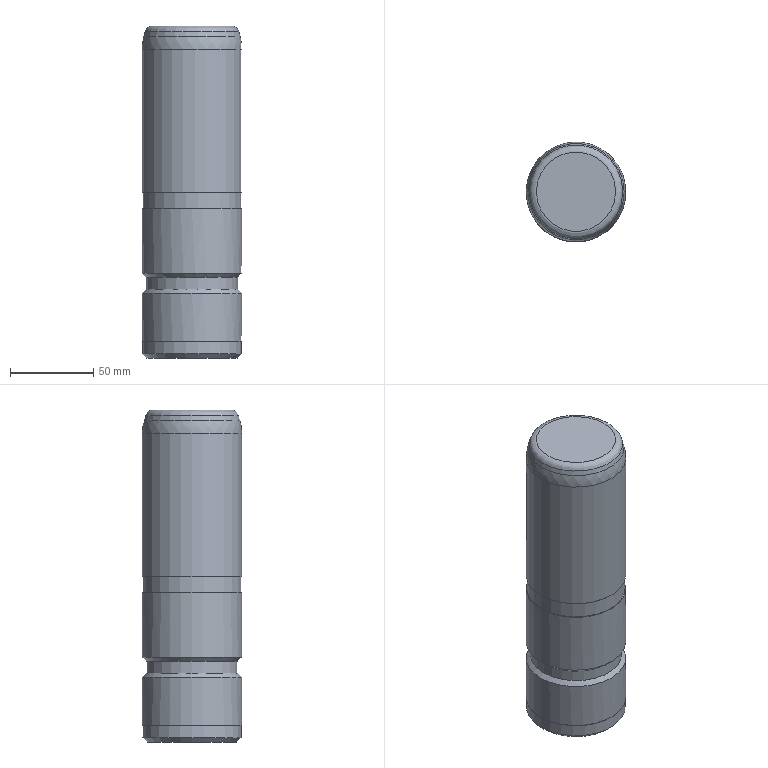Part | NX | features solid 2 | 1 solid | 17 faces | box 60 x 60 x 200 mm | volume 556247 mm3 | cylinder 6 | plane 5 | cone 4 | sphere 1 | torus 1 | commonest cylinder face diameters 60 x3 55 x1 59 x1 59.5 x1
STEP:
#1=CARTESIAN_POINT('',(1295.,185.,-349.));
#2=VERTEX_POINT('',#1);
#3=CARTESIAN_POINT('',(1325.,185.,-349.));
#4=DIRECTION('',(0.,0.,-1.));
#5=DIRECTION('',(-1.,0.,0.));
#6=AXIS2_PLACEMENT_3D('',#3,#4,#5);
#7=CIRCLE('',#6,30.);
#8=EDGE_CURVE('',#2,#2,#7,.F.);
#9=ORIENTED_EDGE('',*,*,#8,.T.);
#10=EDGE_LOOP('',(#9));
#11=FACE_BOUND('',#10,.T.);
#12=CARTESIAN_POINT('',(1355.,185.,-310.));
#13=VERTEX_POINT('',#12);
#14=CARTESIAN_POINT('',(1325.,185.,-310.));
#15=DIRECTION('',(0.,0.,1.));
#16=DIRECTION('',(1.,0.,0.));
#17=AXIS2_PLACEMENT_3D('',#14,#15,#16);
#18=CIRCLE('',#17,30.);
#19=EDGE_CURVE('',#13,#13,#18,.T.);
#20=ORIENTED_EDGE('',*,*,#19,.F.);
#21=EDGE_LOOP('',(#20));
#22=FACE_BOUND('',#21,.T.);
#23=CARTESIAN_POINT('',(1325.,185.,-390.));
#24=DIRECTION('',(0.,0.,1.));
#25=DIRECTION('',(-1.,0.,0.));
#26=AXIS2_PLACEMENT_3D('',#23,#24,#25);
#27=CYLINDRICAL_SURFACE('',#26,30.);
#28=ADVANCED_FACE('',(#11,#22),#27,.T.);
#29=CARTESIAN_POINT('',(1295.5,185.,-310.));
#30=VERTEX_POINT('',#29);
#31=CARTESIAN_POINT('',(1325.,185.,-310.));
#32=DIRECTION('',(0.,0.,-1.));
#33=DIRECTION('',(-1.,0.,0.));
#34=AXIS2_PLACEMENT_3D('',#31,#32,#33);
#35=CIRCLE('',#34,29.5);
#36=EDGE_CURVE('',#30,#30,#35,.T.);
#37=ORIENTED_EDGE('',*,*,#36,.T.);
#38=EDGE_LOOP('',(#37));
#39=FACE_BOUND('',#38,.T.);
#40=ORIENTED_EDGE('',*,*,#19,.T.);
#41=EDGE_LOOP('',(#40));
#42=FACE_BOUND('',#41,.T.);
#43=CARTESIAN_POINT('',(1325.,185.,-310.));
#44=DIRECTION('',(0.,0.,1.));
#45=DIRECTION('',(-1.,0.,0.));
#46=AXIS2_PLACEMENT_3D('',#43,#44,#45);
#47=PLANE('',#46);
#48=ADVANCED_FACE('',(#39,#42),#47,.T.);
#49=CARTESIAN_POINT('',(1354.5,185.,-300.));
#50=VERTEX_POINT('',#49);
#51=CARTESIAN_POINT('',(1325.,185.,-300.));
#52=DIRECTION('',(0.,0.,1.));
#53=DIRECTION('',(1.,0.,0.));
#54=AXIS2_PLACEMENT_3D('',#51,#52,#53);
#55=CIRCLE('',#54,29.5);
#56=EDGE_CURVE('',#50,#50,#55,.F.);
#57=ORIENTED_EDGE('',*,*,#56,.T.);
#58=EDGE_LOOP('',(#57));
#59=FACE_BOUND('',#58,.T.);
#60=ORIENTED_EDGE('',*,*,#36,.F.);
#61=EDGE_LOOP('',(#60));
#62=FACE_BOUND('',#61,.T.);
#63=CARTESIAN_POINT('',(1325.,185.,-310.));
#64=DIRECTION('',(0.,0.,1.));
#65=DIRECTION('',(-1.,0.,0.));
#66=AXIS2_PLACEMENT_3D('',#63,#64,#65);
#67=CYLINDRICAL_SURFACE('',#66,29.5);
#68=ADVANCED_FACE('',(#59,#62),#67,.T.);
#69=ORIENTED_EDGE('',*,*,#56,.F.);
#70=EDGE_LOOP('',(#69));
#71=FACE_BOUND('',#70,.T.);
#72=CARTESIAN_POINT('',(1295.,185.,-300.));
#73=VERTEX_POINT('',#72);
#74=CARTESIAN_POINT('',(1325.,185.,-300.));
#75=DIRECTION('',(0.,0.,-1.));
#76=DIRECTION('',(-1.,0.,0.));
#77=AXIS2_PLACEMENT_3D('',#74,#75,#76);
#78=CIRCLE('',#77,30.);
#79=EDGE_CURVE('',#73,#73,#78,.T.);
#80=ORIENTED_EDGE('',*,*,#79,.T.);
#81=EDGE_LOOP('',(#80));
#82=FACE_BOUND('',#81,.T.);
#83=CARTESIAN_POINT('',(1325.,185.,-300.));
#84=DIRECTION('',(0.,0.,-1.));
#85=DIRECTION('',(1.,0.,0.));
#86=AXIS2_PLACEMENT_3D('',#83,#84,#85);
#87=PLANE('',#86);
#88=ADVANCED_FACE('',(#71,#82),#87,.T.);
#89=CARTESIAN_POINT('',(1295.,185.,-213.95));
#90=VERTEX_POINT('',#89);
#91=CARTESIAN_POINT('',(1325.,185.,-213.95));
#92=DIRECTION('',(0.,0.,-1.));
#93=DIRECTION('',(-1.,0.,0.));
#94=AXIS2_PLACEMENT_3D('',#91,#92,#93);
#95=CIRCLE('',#94,30.);
#96=EDGE_CURVE('',#90,#90,#95,.F.);
#97=ORIENTED_EDGE('',*,*,#96,.F.);
#98=EDGE_LOOP('',(#97));
#99=FACE_BOUND('',#98,.T.);
#100=ORIENTED_EDGE('',*,*,#79,.F.);
#101=EDGE_LOOP('',(#100));
#102=FACE_BOUND('',#101,.T.);
#103=CARTESIAN_POINT('',(1325.,185.,-300.));
#104=DIRECTION('',(0.,0.,1.));
#105=DIRECTION('',(-1.,0.,0.));
#106=AXIS2_PLACEMENT_3D('',#103,#104,#105);
#107=CYLINDRICAL_SURFACE('',#106,30.);
#108=ADVANCED_FACE('',(#99,#102),#107,.T.);
#109=CARTESIAN_POINT('',(1301.132,185.,-200.));
#110=VERTEX_POINT('',#109);
#111=CARTESIAN_POINT('',(1325.,185.,-200.));
#112=DIRECTION('',(0.,0.,-1.));
#113=DIRECTION('',(-1.,0.,0.));
#114=AXIS2_PLACEMENT_3D('',#111,#112,#113);
#115=CIRCLE('',#114,23.868);
#116=EDGE_CURVE('',#110,#110,#115,.T.);
#117=ORIENTED_EDGE('',*,*,#116,.F.);
#118=EDGE_LOOP('',(#117));
#119=FACE_BOUND('',#118,.T.);
#120=CARTESIAN_POINT('',(1325.,185.,-200.));
#121=DIRECTION('',(0.,0.,1.));
#122=DIRECTION('',(-1.,0.,0.));
#123=AXIS2_PLACEMENT_3D('',#120,#121,#122);
#124=PLANE('',#123);
#125=ADVANCED_FACE('',(#119),#124,.T.);
#126=CARTESIAN_POINT('',(1296.786,185.,-203.335));
#127=VERTEX_POINT('',#126);
#128=CARTESIAN_POINT('',(1325.,185.,-203.335));
#129=DIRECTION('',(0.,0.,-1.));
#130=DIRECTION('',(-1.,0.,0.));
#131=AXIS2_PLACEMENT_3D('',#128,#129,#130);
#132=CIRCLE('',#131,28.214);
#133=EDGE_CURVE('',#127,#127,#132,.F.);
#134=ORIENTED_EDGE('',*,*,#133,.F.);
#135=EDGE_LOOP('',(#134));
#136=FACE_BOUND('',#135,.T.);
#137=CARTESIAN_POINT('',(1353.978,185.,-206.185));
#138=VERTEX_POINT('',#137);
#139=CARTESIAN_POINT('',(1325.,185.,-206.185));
#140=DIRECTION('',(0.,0.,1.));
#141=DIRECTION('',(1.,0.,0.));
#142=AXIS2_PLACEMENT_3D('',#139,#140,#141);
#143=CIRCLE('',#142,28.978);
#144=EDGE_CURVE('',#138,#138,#143,.F.);
#145=ORIENTED_EDGE('',*,*,#144,.F.);
#146=EDGE_LOOP('',(#145));
#147=FACE_BOUND('',#146,.T.);
#148=CARTESIAN_POINT('',(1325.,185.,-200.));
#149=DIRECTION('',(0.,0.,-1.));
#150=DIRECTION('',(1.,0.,0.));
#151=AXIS2_PLACEMENT_3D('',#148,#149,#150);
#152=CONICAL_SURFACE('',#151,27.321,0.2618);
#153=ADVANCED_FACE('',(#136,#147),#152,.T.);
#154=CARTESIAN_POINT('',(1297.5,185.,-351.5));
#155=VERTEX_POINT('',#154);
#156=CARTESIAN_POINT('',(1325.,185.,-351.5));
#157=DIRECTION('',(0.,0.,-1.));
#158=DIRECTION('',(-1.,0.,0.));
#159=AXIS2_PLACEMENT_3D('',#156,#157,#158);
#160=CIRCLE('',#159,27.5);
#161=EDGE_CURVE('',#155,#155,#160,.F.);
#162=ORIENTED_EDGE('',*,*,#161,.F.);
#163=EDGE_LOOP('',(#162));
#164=FACE_BOUND('',#163,.T.);
#165=CARTESIAN_POINT('',(1352.5,185.,-358.5));
#166=VERTEX_POINT('',#165);
#167=CARTESIAN_POINT('',(1325.,185.,-358.5));
#168=DIRECTION('',(0.,0.,1.));
#169=DIRECTION('',(1.,0.,0.));
#170=AXIS2_PLACEMENT_3D('',#167,#168,#169);
#171=CIRCLE('',#170,27.5);
#172=EDGE_CURVE('',#166,#166,#171,.F.);
#173=ORIENTED_EDGE('',*,*,#172,.F.);
#174=EDGE_LOOP('',(#173));
#175=FACE_BOUND('',#174,.T.);
#176=CARTESIAN_POINT('',(1325.,185.,-361.));
#177=DIRECTION('',(0.,0.,1.));
#178=DIRECTION('',(-1.,0.,0.));
#179=AXIS2_PLACEMENT_3D('',#176,#177,#178);
#180=CYLINDRICAL_SURFACE('',#179,27.5);
#181=ADVANCED_FACE('',(#164,#175),#180,.T.);
#182=CARTESIAN_POINT('',(1352.25,185.,-400.));
#183=VERTEX_POINT('',#182);
#184=CARTESIAN_POINT('',(1325.,185.,-400.));
#185=DIRECTION('',(0.,0.,1.));
#186=DIRECTION('',(1.,0.,0.));
#187=AXIS2_PLACEMENT_3D('',#184,#185,#186);
#188=CIRCLE('',#187,27.25);
#189=EDGE_CURVE('',#183,#183,#188,.T.);
#190=ORIENTED_EDGE('',*,*,#189,.F.);
#191=EDGE_LOOP('',(#190));
#192=FACE_BOUND('',#191,.T.);
#193=CARTESIAN_POINT('',(1325.,185.,-400.));
#194=DIRECTION('',(0.,0.,-1.));
#195=DIRECTION('',(1.,0.,0.));
#196=AXIS2_PLACEMENT_3D('',#193,#194,#195);
#197=PLANE('',#196);
#198=ADVANCED_FACE('',(#192),#197,.T.);
#199=CARTESIAN_POINT('',(1354.75,185.,-397.5));
#200=VERTEX_POINT('',#199);
#201=CARTESIAN_POINT('',(1325.,185.,-397.5));
#202=DIRECTION('',(0.,0.,1.));
#203=DIRECTION('',(1.,0.,0.));
#204=AXIS2_PLACEMENT_3D('',#201,#202,#203);
#205=CIRCLE('',#204,29.75);
#206=EDGE_CURVE('',#200,#200,#205,.F.);
#207=ORIENTED_EDGE('',*,*,#206,.F.);
#208=EDGE_LOOP('',(#207));
#209=FACE_BOUND('',#208,.T.);
#210=CARTESIAN_POINT('',(1354.75,185.,-390.));
#211=VERTEX_POINT('',#210);
#212=CARTESIAN_POINT('',(1325.,185.,-390.));
#213=DIRECTION('',(0.,0.,1.));
#214=DIRECTION('',(1.,0.,0.));
#215=AXIS2_PLACEMENT_3D('',#212,#213,#214);
#216=CIRCLE('',#215,29.75);
#217=EDGE_CURVE('',#211,#211,#216,.F.);
#218=ORIENTED_EDGE('',*,*,#217,.T.);
#219=EDGE_LOOP('',(#218));
#220=FACE_BOUND('',#219,.T.);
#221=CARTESIAN_POINT('',(1325.,185.,-400.));
#222=DIRECTION('',(0.,0.,1.));
#223=DIRECTION('',(-1.,0.,0.));
#224=AXIS2_PLACEMENT_3D('',#221,#222,#223);
#225=CYLINDRICAL_SURFACE('',#224,29.75);
#226=ADVANCED_FACE('',(#209,#220),#225,.T.);
#227=ORIENTED_EDGE('',*,*,#217,.F.);
#228=EDGE_LOOP('',(#227));
#229=FACE_BOUND('',#228,.T.);
#230=CARTESIAN_POINT('',(1295.,185.,-390.));
#231=VERTEX_POINT('',#230);
#232=CARTESIAN_POINT('',(1325.,185.,-390.));
#233=DIRECTION('',(0.,0.,-1.));
#234=DIRECTION('',(-1.,0.,0.));
#235=AXIS2_PLACEMENT_3D('',#232,#233,#234);
#236=CIRCLE('',#235,30.);
#237=EDGE_CURVE('',#231,#231,#236,.T.);
#238=ORIENTED_EDGE('',*,*,#237,.T.);
#239=EDGE_LOOP('',(#238));
#240=FACE_BOUND('',#239,.T.);
#241=CARTESIAN_POINT('',(1325.,185.,-390.));
#242=DIRECTION('',(0.,0.,-1.));
#243=DIRECTION('',(1.,0.,0.));
#244=AXIS2_PLACEMENT_3D('',#241,#242,#243);
#245=PLANE('',#244);
#246=ADVANCED_FACE('',(#229,#240),#245,.T.);
#247=CARTESIAN_POINT('',(1355.,185.,-361.));
#248=VERTEX_POINT('',#247);
#249=CARTESIAN_POINT('',(1325.,185.,-361.));
#250=DIRECTION('',(0.,0.,1.));
#251=DIRECTION('',(1.,0.,0.));
#252=AXIS2_PLACEMENT_3D('',#249,#250,#251);
#253=CIRCLE('',#252,30.);
#254=EDGE_CURVE('',#248,#248,#253,.F.);
#255=ORIENTED_EDGE('',*,*,#254,.T.);
#256=EDGE_LOOP('',(#255));
#257=FACE_BOUND('',#256,.T.);
#258=ORIENTED_EDGE('',*,*,#237,.F.);
#259=EDGE_LOOP('',(#258));
#260=FACE_BOUND('',#259,.T.);
#261=CARTESIAN_POINT('',(1325.,185.,-390.));
#262=DIRECTION('',(0.,0.,1.));
#263=DIRECTION('',(-1.,0.,0.));
#264=AXIS2_PLACEMENT_3D('',#261,#262,#263);
#265=CYLINDRICAL_SURFACE('',#264,30.);
#266=ADVANCED_FACE('',(#257,#260),#265,.T.);
#267=ORIENTED_EDGE('',*,*,#189,.T.);
#268=EDGE_LOOP('',(#267));
#269=FACE_BOUND('',#268,.T.);
#270=ORIENTED_EDGE('',*,*,#206,.T.);
#271=EDGE_LOOP('',(#270));
#272=FACE_BOUND('',#271,.T.);
#273=CARTESIAN_POINT('',(1325.,185.,-397.5));
#274=DIRECTION('',(0.,0.,1.));
#275=DIRECTION('',(-1.,0.,0.));
#276=AXIS2_PLACEMENT_3D('',#273,#274,#275);
#277=CONICAL_SURFACE('',#276,29.75,0.7854);
#278=ADVANCED_FACE('',(#269,#272),#277,.T.);
#279=ORIENTED_EDGE('',*,*,#254,.F.);
#280=EDGE_LOOP('',(#279));
#281=FACE_BOUND('',#280,.T.);
#282=ORIENTED_EDGE('',*,*,#172,.T.);
#283=EDGE_LOOP('',(#282));
#284=FACE_BOUND('',#283,.T.);
#285=CARTESIAN_POINT('',(1325.,185.,-358.5));
#286=DIRECTION('',(0.,0.,-1.));
#287=DIRECTION('',(1.,0.,0.));
#288=AXIS2_PLACEMENT_3D('',#285,#286,#287);
#289=CONICAL_SURFACE('',#288,27.5,0.7854);
#290=ADVANCED_FACE('',(#281,#284),#289,.T.);
#291=ORIENTED_EDGE('',*,*,#8,.F.);
#292=EDGE_LOOP('',(#291));
#293=FACE_BOUND('',#292,.T.);
#294=ORIENTED_EDGE('',*,*,#161,.T.);
#295=EDGE_LOOP('',(#294));
#296=FACE_BOUND('',#295,.T.);
#297=CARTESIAN_POINT('',(1325.,185.,-351.5));
#298=DIRECTION('',(0.,0.,1.));
#299=DIRECTION('',(-1.,0.,0.));
#300=AXIS2_PLACEMENT_3D('',#297,#298,#299);
#301=CONICAL_SURFACE('',#300,27.5,0.7854);
#302=ADVANCED_FACE('',(#293,#296),#301,.T.);
#303=ORIENTED_EDGE('',*,*,#96,.T.);
#304=EDGE_LOOP('',(#303));
#305=FACE_BOUND('',#304,.T.);
#306=ORIENTED_EDGE('',*,*,#144,.T.);
#307=EDGE_LOOP('',(#306));
#308=FACE_BOUND('',#307,.T.);
#309=CARTESIAN_POINT('',(1325.,185.,-213.95));
#310=DIRECTION('',(0.,0.,1.));
#311=DIRECTION('',(-1.,0.,0.));
#312=AXIS2_PLACEMENT_3D('',#309,#310,#311);
#313=SPHERICAL_SURFACE('',#312,30.);
#314=ADVANCED_FACE('',(#305,#308),#313,.T.);
#315=ORIENTED_EDGE('',*,*,#116,.T.);
#316=EDGE_LOOP('',(#315));
#317=FACE_BOUND('',#316,.T.);
#318=ORIENTED_EDGE('',*,*,#133,.T.);
#319=EDGE_LOOP('',(#318));
#320=FACE_BOUND('',#319,.T.);
#321=CARTESIAN_POINT('',(1325.,185.,-204.5));
#322=DIRECTION('',(0.,0.,1.));
#323=DIRECTION('',(-1.,0.,0.));
#324=AXIS2_PLACEMENT_3D('',#321,#322,#323);
#325=TOROIDAL_SURFACE('',#324,23.868,4.5);
#326=ADVANCED_FACE('',(#317,#320),#325,.T.);
#327=CLOSED_SHELL('',(#28,#48,#68,#88,#108,#125,#153,#181,#198,#226,#246,#266,#278,#290,#302,#314,#326));
#328=MANIFOLD_SOLID_BREP('',#327);
#329=(LENGTH_UNIT()NAMED_UNIT(*)SI_UNIT(.MILLI.,.METRE.));
#330=UNCERTAINTY_MEASURE_WITH_UNIT(LENGTH_MEASURE(0.00001),#329,'','');
#331=(NAMED_UNIT(*)PLANE_ANGLE_UNIT()SI_UNIT($,.RADIAN.));
#332=(NAMED_UNIT(*)SI_UNIT($,.STERADIAN.)SOLID_ANGLE_UNIT());
#333=(GEOMETRIC_REPRESENTATION_CONTEXT(3)GLOBAL_UNCERTAINTY_ASSIGNED_CONTEXT((#330))GLOBAL_UNIT_ASSIGNED_CONTEXT((#329,#331,#332))REPRESENTATION_CONTEXT('',''));
#334=ADVANCED_BREP_SHAPE_REPRESENTATION('',(#328),#333);